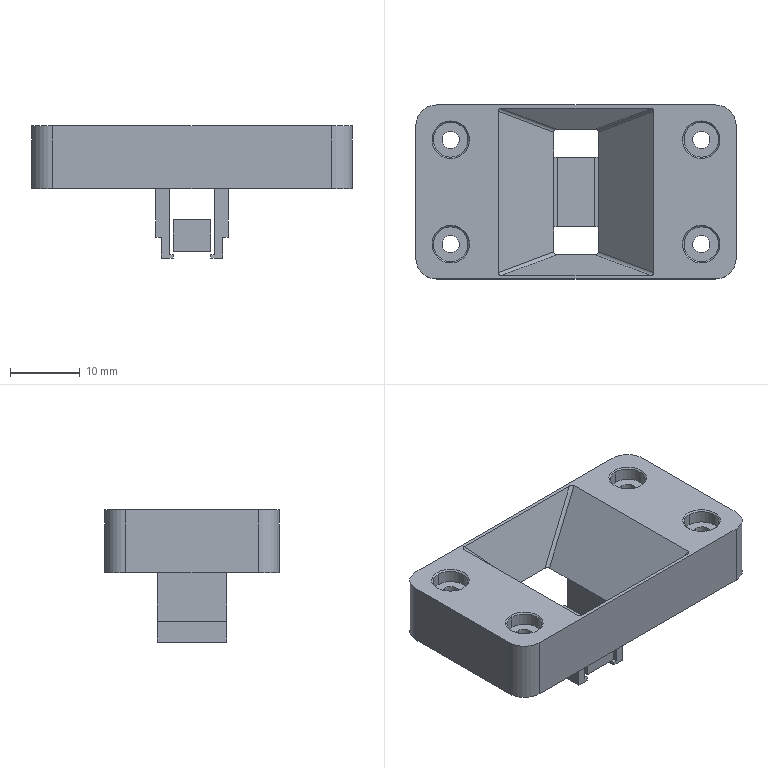NC program | NX | posted with a generic post | part box 46 x 25 x 19 mm
Whole program:
N10 G17 G21 G94 G90
(FLOOR_WALL_COPY , TOOL : D63)
N12 T01 M6
N14 G54
N16 G17 G0 G90 X57.5 Y0. S6500 M3
N18 G43 Z30. H1
N20 Z8.
N22 G94 G1 Z5. F1250.
N24 X54.5
N26 X-54.5
N28 X-57.5
N30 Z8.
N32 G0 Z30.
N34 X57.5
N36 Z7.
N38 G1 Z4.
N40 X54.5
N42 X-54.5
N44 X-57.5
N46 Z7.
N48 G0 Z30.
N50 X57.5
N52 Z6.
N54 G1 Z3.
N56 X54.5
N58 X-54.5
N60 X-57.5
N62 Z6.
N64 G0 Z30.
N66 X57.5
N68 Z5.
N70 G1 Z2.
N72 X54.5
N74 X-54.5
N76 X-57.5
N78 Z5.
N80 G0 Z30.
N82 X57.5
N84 Z4.
N86 G1 Z1.
N88 X54.5
N90 X-54.5
N92 X-57.5
N94 Z4.
N96 G0 Z30.
N98 X57.5
N100 Z3.
N102 G1 Z0.
N104 X54.5
N106 X-54.5
N108 X-57.5
N110 Z3.
N112 G0 Z30.
N114 M5
(ADAPTIVE_MILLING_COPY , TOOL : D10)
N116 T10 M6
N118 G54
N120 G17 G0 G90 X10.349 Y20.195 S9500 M3
N122 G43 Z30. H10
N124 Z-8.85
N126 G94 G1 Z-9.85 F1000.
N128 X9.819 Y18.839 F3000.
N130 G3 X10.349 Y17.549 R1.015
N132 X13.508 Y16.905 R9.424
N134 X20.803 Y16.691 R188.288
N136 G2 X25.145 Y13.62 R6.148
N138 X26.85 Y8.021 R13.627
N140 X27.174 Y-0.369 R83.294
N142 X27.162 Y-10.268 R643.501
N144 X24.292 Y-14.521 R6.049
N146 X18.726 Y-16.321 R13.096
N148 X10.138 Y-16.674 R78.513
N150 G1 X8.738 Y-16.68
N152 X6.738 Y-16.685
N154 X3.338 Y-16.688
N156 X-7.562 Y-16.689
N158 X-20.262
N160 X-20.362
N162 G2 X-24.729 Y-14.206 R5.74
N164 X-26.754 Y-8.729 R11.979
N166 X-27.166 Y-0.746 R62.374
N168 G1 X-27.174 Y0.354
N170 X-27.181 Y1.854
N172 X-27.185 Y3.954
N174 X-27.188 Y7.554
N176 X-27.189 Y9.754
N178 X-27.188 Y9.854
N180 X-27.186 Y9.954
N182 X-27.181 Y10.054
N184 X-27.173 Y10.154
N186 X-27.165 Y10.253
N188 G2 X-24.303 Y14.512 R6.044
N190 X-18.74 Y16.32 R13.03
N192 X-9.952 Y16.675 R80.043
N194 X7.847 Y16.662 R941.417
N196 G3 X16.12 Y16.025 R146.197
N198 G2 X19.397 Y15.731 R13.879
N200 X24.449 Y11.335 R8.19
N202 X26.087 Y4.777 R18.158
N204 X26.337 Y-7.815 R137.782
N206 X22.284 Y-13.67 R7.754
N208 X15.993 Y-15.506 R16.182
N210 X6.504 Y-15.865 R95.225
N212 G1 X5.004 Y-15.871
N214 X2.804 Y-15.877
N216 X-0.896 Y-15.88
N218 X-12.396 Y-15.881
N220 X-17.496
N222 X-17.696 Y-15.879
N224 G2 X-24.003 Y-12.063 R7.592
N226 X-25.967 Y-5.816 R15.383
N228 X-26.364 Y3.87 R86.818
N230 X-26.307 Y8.067 R42.038
N232 X-22.239 Y13.697 R7.801
N234 X-15.941 Y15.513 R16.361
N236 X-5.851 Y15.868 R103.703
N238 X6.748 Y15.835 R488.212
N240 G1 X7.147 Y15.815
N242 X7.447 Y15.797
N244 X7.946 Y15.765
N246 X8.544 Y15.723
N248 X9.342 Y15.662
N250 X10.139 Y15.599
N252 X10.838 Y15.548
N254 X11.935 Y15.471
N256 X12.833 Y15.411
N258 X13.532 Y15.372
N260 X14.231 Y15.336
N262 X14.93 Y15.304
N264 X15.33 Y15.286
N266 X15.629 Y15.27
N268 X15.829 Y15.256
N270 X15.929 Y15.249
N272 X16.128 Y15.23
N274 X16.327 Y15.209
N276 X16.426 Y15.198
N278 G2 X23.41 Y10.123 R9.068
N280 X25.231 Y3.1 R19.368
N282 X25.483 Y-5.99 R67.248
N284 X20.853 Y-12.719 R8.758
N286 X14.175 Y-14.657 R17.662
N288 X3.888 Y-15.055 R99.931
N290 G1 X2.188 Y-15.062
N292 X-0.012 Y-15.067
N294 X-3.612 Y-15.071
N296 X-13.112 Y-15.072
N298 X-15.212
N300 X-15.412 Y-15.069
N302 G2 X-23.226 Y-10.35 R8.79
N304 X-25.195 Y-3.372 R18.115
N306 X-25.489 Y5.916 R69.639
N308 X-20.831 Y12.732 R8.743
N310 X-13.951 Y14.683 R17.964
N312 X-2.962 Y15.059 R115.566
N314 X8.234 Y14.898 R167.957
N316 X14.818 Y14.461 R201.47
N318 X22.586 Y8.699 R9.966
N320 X24.372 Y1.763 R20.573
N322 X24.594 Y-4.426 R36.555
N324 X19.388 Y-11.896 R9.487
N326 X12.298 Y-13.851 R19.437
N328 X1.91 Y-14.244 R108.047
N330 X-14.19 Y-14.234 R840.622
N332 X-22.416 Y-8.882 R9.633
N334 X-24.357 Y-1.787 R19.688
N336 X-24.593 Y4.4 R36.405
N338 X-19.407 Y11.885 R9.484
N340 X-12.618 Y13.811 R18.928
N342 X-1.632 Y14.246 R105.155
N344 X13.252 Y13.729 R140.906
N346 X21.72 Y7.49 R10.666
N348 X23.596 Y-0.242 R22.348
N350 X22.778 Y-6.31 R11.45
N352 X17.076 Y-11.518 R10.761
N354 X9.483 Y-13.146 R24.225
N356 X-3.611 Y-13.448 R188.91
N358 X-12.91 Y-13.399 R239.93
N360 X-21.646 Y-7.451 R10.299
N362 X-23.544 Y-0.134 R21.268
N364 X-23.071 Y5.592 R12.411
N366 X-17.418 Y11.366 R10.417
N368 X-10.253 Y13.078 R22.555
N370 X2.937 Y13.423 R139.477
N372 X12.021 Y12.956 R98.72
N374 X20.845 Y6.384 R11.22
N376 X22.561 Y-2.057 R17.672
N378 X17.27 Y-9.947 R10.011
N380 X9.839 Y-12.14 R19.815
N382 X-0.045 Y-12.61 R92.479
N384 X-11.244 Y-12.597 R330.002
N386 X-20.849 Y-6.145 R10.877
N388 X-22.539 Y2.097 R17.102
N390 X-17.313 Y9.918 R9.956
N392 X-9.988 Y12.122 R19.589
N394 X2.495 Y12.597 R100.153
N396 X10.682 Y12.198 R84.458
N398 X20.065 Y5.14 R11.717
N400 X21.305 Y-1.758 R12.728
N402 X16.27 Y-8.958 R9.978
N404 X8.974 Y-11.255 R19.408
N406 X-1.106 Y-11.793 R85.239
N408 X-10.104 Y-11.764 R170.612
N410 X-19.987 Y-5.033 R11.304
N412 X-21.243 Y1.951 R12.259
N414 X-16.336 Y8.908 R9.934
N416 X-9.054 Y11.243 R19.216
N418 X3.625 Y11.749 R87.295
N420 X10.301 Y11.284 R43.324
N422 X20.037 Y0.334 R11.84
N424 X15.863 Y-7.551 R9.385
N426 X8.824 Y-10.248 R17.2
N428 X-0.841 Y-10.956 R64.727
N430 X-9.138 Y-10.919 R105.066
N432 X-19.946 Y-0.58 R11.432
N434 X-16.016 Y7.416 R9.231
N436 X-9.117 Y10.189 R16.617
N438 X1.143 Y10.931 R59.23
N440 X8.826 Y10.557 R50.308
N442 X17.793 Y3.975 R11.631
N444 X15.558 Y-5.864 R8.534
N446 X8.899 Y-9.132 R14.655
N448 G3 X7.711 Y-9.486 R3.375
N450 G2 X5.166 Y-10.15 R6.048
N452 X-7.034 Y-10.148 R858.46
N454 X-14.111 Y-8.012 R12.901
N456 X-18.319 Y-1.582 R9.717
N458 X-15.184 Y6.138 R8.589
N460 X-8.435 Y9.229 R15.191
N462 G3 X-7.711 Y9.486 R2.216
N464 G2 X-5.166 Y10.15 R6.048
N466 G1 X5.166
N468 X5.234 Y10.146
N470 G2 X11.238 Y8.735 R17.863
N472 X16.254 Y3.799 R9.75
N474 X14.554 Y-4.542 R7.842
N476 X9.732 Y-7.679 R13.426
N478 G3 X8.883 Y-8.587 R2.865
N480 G1 X8.787 Y-8.683
N482 X7.835 Y-9.414
N484 G2 X5.166 Y-10.15 R6.017
N486 G1 X-3.034
N488 G2 X-6.597 Y-9.948 R15.885
N490 X-10.87 Y-8.552 R40.547
N492 X-15.862 Y-4.131 R9.949
N494 X-14.551 Y4.421 R7.639
N496 X-9.781 Y7.631 R13.031
N498 G3 X-8.883 Y8.587 R2.901
N500 G1 X-8.787 Y8.683
N502 X-7.835 Y9.414
N504 G3 X-7.871 Y11.027 R1.003
N506 X-8.777 Y11.17 Z-9.803 R1.146
N508 G1 X-9.821 Y11.019 Z-9.75
N510 X-10.869 Y10.873
N512 X-11.915 Y10.704
N514 X-12.182 Y10.579
N516 X-14.178 Y9.234
N518 G3 X-16.48 Y7.04 R12.484
N520 G1 X-17.127 Y6.24
N522 X-17.734 Y5.41
N524 G3 X-19.277 Y1.86 R11.715
N526 X-19.624 Y-2.353 R12.075
N528 X-16.268 Y-8.781 R10.158
N530 X-14.097 Y-10.294 R11.142
N532 G1 X-10.494 Y-12.198
N534 G3 X-9.883 Y-12.304 R1.044
N536 G1 X-8.099 Y-12.045
N538 X-6.694 Y-11.831 Z-9.821
N540 G3 X-6.216 Y-11.519 Z-9.85 R1.052
N542 X-6.597 Y-9.948 R1.003
N544 G2 X-8.86 Y-8.804 R11.551
N546 X-12.787 Y-6.08 R15.49
N548 X-13.313 Y3.004 R7.028
N550 X-10.445 Y5.919 R17.625
N552 G3 X-10.148 Y6.397 R2.026
N554 G2 X-9.375 Y7.947 R5.18
N556 G3 X-9.767 Y9.472 R1.003
N558 X-10.715 Y9.413 Z-9.801 R1.127
N560 G1 X-11.658 Y9.031 Z-9.75
N562 X-12.609 Y8.653
N564 X-13.552 Y8.253
N566 X-13.728 Y8.115
N568 X-13.875 Y7.947
N570 X-16.301 Y4.307
N572 G3 X-17.769 Y-2.767 R9.618
N574 G1 X-17.6 Y-3.666
N576 X-17.376 Y-4.553
N578 G3 X-15.03 Y-8.116 R7.888
N580 G1 X-12.176 Y-10.583
N582 G3 X-11.646 Y-10.819 R1.05
N584 G1 X-9.83 Y-11.045
N586 X-8.418 Y-11.211 Z-9.821
N588 G3 X-7.875 Y-11.038 Z-9.85 R1.052
N590 X-7.83 Y-9.418 R1.003
N592 G2 X-10.346 Y-7.223 R25.373
N594 X-12.084 Y1.423 R7.16
N596 X-10.425 Y4.388 R49.729
N598 G3 X-10.158 Y6.361 R33.573
N600 X-10.845 Y7.58 R1.005
N602 X-11.845 Y7.337 Z-9.796 R1.11
N604 G1 X-12.607 Y6.81 Z-9.75
N606 X-13.417 Y6.256
N608 X-14.215 Y5.686
N610 G3 X-14.504 Y5.197 R1.052
N612 G1 X-15.759 Y0.176
N614 G3 X-15.8 Y-4.345 R9.728
N616 G1 X-15.484 Y-5.644
N618 G3 X-14.33 Y-7.598 R5.058
N620 G1 X-13.286 Y-8.676
N622 X-13.06 Y-8.812
N624 X-11.273 Y-9.591
N626 X-10.598 Y-9.892 Z-9.787
N628 X-9.912 Y-10.168 Z-9.824
N630 G3 X-9.397 Y-10.156 Z-9.85 R1.113
N632 X-8.883 Y-8.587 R1.002
N634 G2 X-11.272 Y-3.038 R9.813
N636 X-10.405 Y1.852 R12.701
N638 G1 X-10.377 Y1.948
N640 X-10.358 Y2.046
N642 X-10.35 Y2.121
N644 Y4.721
N646 G3 X-12.548 Y4.657 R-1.1
N648 G1 X-11.801 Y-7.997
N650 G3 X-9.686 Y-7.511 R-1.1
N652 G2 X-10.361 Y-4.666 R6.218
N654 G1 X-10.367 Y-4.366
N656 X-10.368 Y-4.066
N658 X-10.365 Y-3.866
N660 X-10.361 Y-3.666
N662 X-10.353 Y-3.466
N664 X-10.35 Y-3.394
N666 Y2.206
N668 G3 X-11.452 Y3.304 R1.1
N670 X-12.55 Y2.206 R1.1
N672 G1 Y-4.966
N674 G3 X-11.448 Y-6.064 R1.1
N676 X-10.35 Y-4.966 R1.1
N678 G1 Y-3.366
N680 G3 X-10.798 Y-2.532 R1.014
N682 G1 X-11.176 Y-2.281
N684 X-12.844 Y-1.177 Z-9.75
N686 X-13.1 Y-1.006
N688 X-13.324 Y-0.795
N690 G2 X-13.532 Y-0.184 R1.041
N692 G1 X-13.537 Y2.523
N694 X-13.521 Y5.229
N696 G2 X-11.306 Y10.454 R8.457
N698 X-9.107 Y12.137 R10.747
N700 X-6.505 Y12.956 R7.004
N702 X-0.909 Y13.305 R53.423
N704 G1 X2.052 Y13.327
N706 G2 X2.874 Y12.908 R1.015
N708 G1 X3.046 Y12.667
N710 X4.207 Y11.038 Z-9.85
N712 X4.656 Y10.431
N714 G3 X5.234 Y10.146 R1.041
N716 G2 X7.982 Y9.358 R6.394
N718 X12.446 Y6.731 R17.201
N720 X13.403 Y-3.093 R7.139
N722 X10.406 Y-6.02 R18.422
N724 G1 X10.337 Y-6.092
N726 X10.274 Y-6.17
N728 X10.218 Y-6.253
N730 X10.169 Y-6.34
N732 X10.16 Y-6.353
N734 X10.148 Y-6.397
N736 G2 X9.375 Y-7.947 R5.18
N738 G3 X9.767 Y-9.472 R1.003
N740 X10.715 Y-9.413 Z-9.801 R1.127
N742 G1 X11.658 Y-9.031 Z-9.75
N744 X12.609 Y-8.653
N746 X13.552 Y-8.253
N748 X13.728 Y-8.115
N750 X13.875 Y-7.947
N752 X15.09 Y-6.133
N754 X16.285 Y-4.305
N756 G3 X17.855 Y-0.3 R13.116
N758 G1 X18.173 Y1.269
N760 G3 X17.902 Y3.829 R5.549
N762 X16.755 Y6.169 R10.806
N764 X14.429 Y9.066 R13.881
N766 G1 X11.609 Y11.736
N768 G3 X10.685 Y11.982 R1.014
N770 G1 X9.091 Y11.595
N772 X8.45 Y11.445 Z-9.783
N774 X7.814 Y11.27 Z-9.816
N776 G3 X7.325 Y10.815 Z-9.85 R1.039
N778 X7.711 Y9.486 R1.005
N780 G2 X11.321 Y6.424 R24.914
N782 X12.313 Y-1.25 R7.01
N784 X10.453 Y-4.444 R31.5
N786 G3 X10.346 Y-5.034 R2.293
N788 G1 X10.184 Y-6.265
N790 X10.158 Y-6.361
N792 G3 X10.846 Y-7.581 R1.005
N794 X11.845 Y-7.337 Z-9.796 R1.11
N796 G1 X12.608 Y-6.809 Z-9.75
N798 X13.417 Y-6.253
N800 X14.216 Y-5.683
N802 G3 X14.504 Y-5.197 R1.053
N804 G1 X15.203 Y-2.474
N806 X15.877 Y0.255
N808 G3 X15.832 Y4.889 R11.427
N810 X14.308 Y8.318 R8.082
N812 G1 X13.134 Y9.848
N814 G3 X12.393 Y10.238 R1.024
N816 G1 X10.695 Y10.328
N818 X10.037 Y10.368 Z-9.783
N820 X9.377 Y10.384 Z-9.816
N822 G3 X8.778 Y10.089 Z-9.85 R1.039
N824 X8.787 Y8.683 R1.005
N826 G2 X11.225 Y4.215 R10.52
N828 X10.715 Y-1.19 R9.97
N830 G1 X10.35 Y-2.359
N832 Y-4.859
N834 G3 X12.548 Y-4.785 R-1.1
N836 G1 X11.668 Y8.254
N838 G3 X9.618 Y7.63 R-1.1
N840 G2 X10.346 Y5.034 R5.902
N842 X10.35 Y2.7 R20.133
N844 G1 Y-2.4
N846 G3 X11.452 Y-3.498 R1.1
N848 X12.55 Y-2.4 R1.1
N850 G1 Y4.966
N852 G3 X11.448 Y6.064 R1.1
N854 X10.35 Y4.966 R1.1
N856 G1 Y2.666
N858 G3 X11.321 Y1.656 R1.015
N860 G1 X12.734 Y1.602
N862 Z-6.85
N864 G0 Z30.
N866 X3.864 Y12.65
N868 Z-1.85
N870 G1 Z-2.85 F1000.
N872 X4.09 Y10.945 F3000.
N874 G3 X4.959 Y10.076 R1.017
N876 G2 X7.03 Y9.418 R5.157
N878 X9.384 Y6.265 R5.459
N880 G1 X9.546 Y5.034
N882 X9.55 Y4.966
N884 Y-4.966
N886 X9.546 Y-5.034
N888 G2 X8.083 Y-8.587 R5.543
N890 X5.665 Y-9.984 R5.703
N892 G1 X4.872 Y-10.088
N894 G3 X4.004 Y-10.944 R1.017
N896 G1 X3.756 Y-12.646
N898 Z0.15
N900 G0 Z30.
N902 X-3.791 Y-12.65
N904 Z-1.85
N906 G1 Z-2.85 F1000.
N908 X-4.032 Y-10.944 F3000.
N910 G3 X-4.9 Y-10.084 R1.017
N912 G2 X-7.03 Y-9.418 R5.213
N914 X-9.384 Y-6.265 R5.459
N916 G1 X-9.546 Y-5.034
N918 X-9.55 Y-4.966
N920 Y4.966
N922 X-9.546 Y5.034
N924 G2 X-8.083 Y8.587 R5.543
N926 X-5.665 Y9.984 R5.703
N928 G1 X-4.872 Y10.088
N930 G3 X-4.004 Y10.944 R1.017
N932 G1 X-3.756 Y12.646
N934 Z0.15
N936 G0 Z30.
N938 M5
(FLOOR_WALL_1 , TOOL : D6)
N940 T06 M6
N942 G54
N944 G17 G0 G90 X9.322 Y8.996 S9500 M3
N946 G43 Z30. H6
N948 Z-1.5
N950 G94 G1 Z-3. F1250.
N952 X8.497 Y8.52
N954 G3 X8.197 Y8. R0.6
N956 G1 Y-8.
N958 X7.7
N960 Y8.
N962 G2 X8. Y8.52 R0.6
N964 G1 X9.134 Y9.174
N966 Z-1.5
N968 G0 Z30.
N970 X8.999 Y9.27
N972 Z-1.5
N974 G1 Z-3.
N976 X7.7 Y8.52
N978 G3 X7.4 Y8. R0.6
N980 G1 Y-8.
N982 G3 X7.7 Y-8.52 R0.6
N984 G1 X8.999 Y-9.27
N986 Z-1.5
N988 G0 Z30.
N990 X21.216 Y-16.901
N992 Z-8.5
N994 G1 Z-10.
N996 X20.58 Y-15.8
N998 G3 X20.061 Y-15.5 R0.6
N1000 G1 X14.75
N1002 X-20.
N1004 G2 X-25.102 Y-12.658 R6.
N1006 G1 X25.104 Y-12.655
N1008 G3 X25.992 Y-9.81 R6.
N1010 G1 X-25.992 Y-9.813
N1012 G2 X-26. Y-9.5 R6.
N1014 G1 Y-6.968
N1016 X-8.5 Y-6.967
N1018 Y-4.123
N1020 X-26. Y-4.124
N1022 Y-1.279
N1024 X-8.5 Y-1.278
N1026 Y1.566
N1028 X-26. Y1.565
N1030 Y4.41
N1032 X-8.5 Y4.411
N1034 Y7.256
N1036 X-26. Y7.255
N1038 G3 X-26.52 Y6.955 R0.6
N1040 G1 X-27.5 Y5.256
N1042 Z-8.5
N1044 G0 Z30.
N1046 X-8.5 Y-6.967
N1048 Z-8.5
N1050 G1 Z-10.
N1052 Y-8.
N1054 G3 X-8.2 Y-8.3 R0.3
N1056 G1 X8.2
N1058 G3 X8.5 Y-8. R0.3
N1060 G1 Y-6.966
N1062 X26. Y-6.965
N1064 Y-4.121
N1066 X8.5 Y-4.122
N1068 Y-1.277
N1070 X26. Y-1.276
N1072 Y1.568
N1074 X8.5 Y1.567
N1076 Y4.412
N1078 X26. Y4.413
N1080 Y7.258
N1082 X8.5 Y7.257
N1084 G3 X8.8 Y6.737 R0.6
N1086 G1 Z-8.5
N1088 G0 Z30.
N1090 X-27.5 Y8.049
N1092 Z-8.5
N1094 G1 Z-10.
N1096 X-26.49 Y9.799
N1098 G2 X-25.97 Y10.099 R0.6
N1100 G1 X25.97 Y10.102
N1102 G2 X26.489 Y9.802 R0.6
N1104 G1 X27.5 Y8.052
N1106 Z-8.5
N1108 G0 Z30.
N1110 X10. Y1.386
N1112 Z-8.5
N1114 G1 Z-10.
N1116 X8.5 Y0.52
N1118 G3 X8.2 Y0. R0.6
N1120 G1 Y-8.
N1122 X-8.2
N1124 Y8.
N1126 X8.2
N1128 Y0.
N1130 G3 X8.5 Y-0.52 R0.6
N1132 G1 X10. Y-1.386
N1134 Z-8.5
N1136 G0 Z30.
N1138 X-9.322 Y-8.996
N1140 Z-1.5
N1142 G1 Z-3.
N1144 X-8.497 Y-8.52
N1146 G3 X-8.197 Y-8. R0.6
N1148 G1 Y8.
N1150 X-7.7
N1152 Y-8.
N1154 G2 X-8. Y-8.52 R0.6
N1156 G1 X-9.134 Y-9.174
N1158 Z-1.5
N1160 G0 Z30.
N1162 X-8.999 Y-9.27
N1164 Z-1.5
N1166 G1 Z-3.
N1168 X-7.7 Y-8.52
N1170 G3 X-7.4 Y-8. R0.6
N1172 G1 Y8.
N1174 G3 X-7.7 Y8.52 R0.6
N1176 G1 X-8.999 Y9.27
N1178 Z-1.5
N1180 G0 Z30.
N1182 M5
(ZLEVEL_PROFILE_1_COPY_1_COPY , TOOL : D6A45)
N1184 T07 M6
N1186 G54
N1188 G17 G0 G90 X-0.75 Y5.92 S9500 M3
N1190 G43 Z30. H7
N1192 Z0.
N1194 G94 G1 Z-1. F1000.
N1196 X-1.444 Y5.519
N1198 G3 X-1.744 Y4.999 R0.6
N1200 G1 Y-4.999
N1202 G2 X-2.699 Y-5.956 R0.956
N1204 G1 X-4.401
N1206 G2 X-5.356 Y-5.001 R0.955
N1208 G1 Y5.001
N1210 G2 X-4.401 Y5.956 R0.955
N1212 G1 X-2.699
N1214 G2 X-1.744 Y4.999 R0.956
N1216 G3 X-1.444 Y4.48 R0.6
N1218 G1 X-0.544 Y3.959
N1220 Z0.
N1222 G0 Z30.
N1224 X0.75 Y-5.92
N1226 Z0.
N1228 G1 Z-1.
N1230 X1.444 Y-5.519
N1232 G3 X1.744 Y-4.999 R0.6
N1234 G1 Y4.999
N1236 G2 X2.699 Y5.956 R0.956
N1238 G1 X4.401
N1240 G2 X5.356 Y5.001 R0.955
N1242 G1 Y-5.001
N1244 G2 X4.401 Y-5.956 R0.955
N1246 G1 X2.699
N1248 G2 X1.744 Y-4.999 R0.956
N1250 G3 X1.444 Y-4.48 R0.6
N1252 G1 X0.544 Y-3.959
N1254 Z0.
N1256 G0 Z30.
(ZLEVEL_PROFILE_1_COPY_1_COPY_COPY , TOOL : D6A45)
N1258 X18.291 Y-7.5
N1260 Z-9.
N1262 G1 Z-11.
N1264 G3 X18. Y-7.209 R0.291
N1266 X18.291 Y-7.5 R-0.291
N1268 X18.141 Y-7.24 R0.3
N1270 G1 Z-10.
N1272 G0 Z30.
N1274 X-18.291 Y7.5
N1276 Z-9.
N1278 G1 Z-11.
N1280 G3 X-18. Y7.209 R0.291
N1282 X-18.291 Y7.5 R-0.291
N1284 X-18.141 Y7.24 R0.3
N1286 G1 Z-10.
N1288 G0 Z30.
N1290 X-18. Y-7.791
N1292 Z-9.
N1294 G1 Z-11.
N1296 X-17.997
N1298 G3 X-17.709 Y-7.497 R0.291
N1300 X-18. Y-7.791 R-0.291
N1302 X-17.74 Y-7.641 R0.3
N1304 G1 Z-10.
N1306 G0 Z30.
N1308 X18. Y7.791
N1310 Z-9.
N1312 G1 Z-11.
N1314 G3 X17.709 Y7.5 R0.291
N1316 X18. Y7.791 R-0.291
N1318 X17.74 Y7.641 R0.3
N1320 G1 Z-10.
N1322 G0 Z30.
N1324 X-20.984 Y14.564
N1326 Z-10.
N1328 G1 Z-11.
N1330 X-20.52 Y13.759
N1332 G3 X-20. Y13.459 R0.6
N1334 G1 X20.
N1336 G2 X23.959 Y9.5 R3.959
N1338 G1 Y-9.5
N1340 G2 X20. Y-13.459 R3.959
N1342 G1 X-20.
N1344 G2 X-23.959 Y-9.5 R3.959
N1346 G1 Y9.5
N1348 G2 X-20. Y13.459 R3.959
N1350 G3 X-19.48 Y13.759 R0.6
N1352 G1 X-18.961 Y14.659
N1354 Z-10.
N1356 G0 Z30.
N1358 M5
N1360 M2